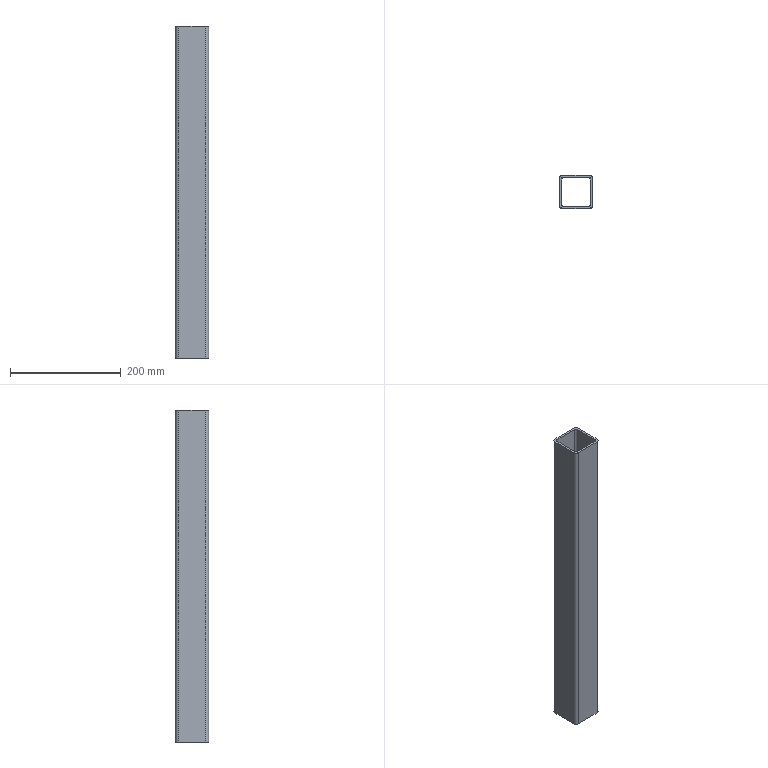Part | SolidWorks | features Fillet 2, Extrusion 1 | 1 solid | 18 faces | box 60 x 60 x 600 mm | volume 523694 mm3 | plane 10 | cylinder 8 | commonest cylinder face diameters 6 x4 12 x4
STEP:
#1=CARTESIAN_POINT('',(-24.,-30.,600.));
#2=VERTEX_POINT('',#1);
#3=CARTESIAN_POINT('',(24.,-30.,600.));
#4=VERTEX_POINT('',#3);
#5=CARTESIAN_POINT('',(-30.,-30.,600.));
#6=DIRECTION('',(1.,0.,0.));
#7=VECTOR('',#6,1000.);
#8=LINE('',#5,#7);
#9=EDGE_CURVE('',#2,#4,#8,.T.);
#10=ORIENTED_EDGE('',*,*,#9,.T.);
#11=CARTESIAN_POINT('',(30.,-24.,600.));
#12=VERTEX_POINT('',#11);
#13=CARTESIAN_POINT('',(24.,-24.,600.));
#14=DIRECTION('',(0.,0.,1.));
#15=DIRECTION('',(-1.,0.,0.));
#16=AXIS2_PLACEMENT_3D('',#13,#14,#15);
#17=CIRCLE('',#16,6.);
#18=EDGE_CURVE('',#4,#12,#17,.T.);
#19=ORIENTED_EDGE('',*,*,#18,.T.);
#20=CARTESIAN_POINT('',(30.,24.,600.));
#21=VERTEX_POINT('',#20);
#22=CARTESIAN_POINT('',(30.,-30.,600.));
#23=DIRECTION('',(0.,1.,0.));
#24=VECTOR('',#23,1000.);
#25=LINE('',#22,#24);
#26=EDGE_CURVE('',#12,#21,#25,.T.);
#27=ORIENTED_EDGE('',*,*,#26,.T.);
#28=CARTESIAN_POINT('',(24.,30.,600.));
#29=VERTEX_POINT('',#28);
#30=CARTESIAN_POINT('',(24.,24.,600.));
#31=DIRECTION('',(0.,0.,1.));
#32=DIRECTION('',(-1.,0.,0.));
#33=AXIS2_PLACEMENT_3D('',#30,#31,#32);
#34=CIRCLE('',#33,6.);
#35=EDGE_CURVE('',#21,#29,#34,.T.);
#36=ORIENTED_EDGE('',*,*,#35,.T.);
#37=CARTESIAN_POINT('',(-24.,30.,600.));
#38=VERTEX_POINT('',#37);
#39=CARTESIAN_POINT('',(-30.,30.,600.));
#40=DIRECTION('',(-1.,0.,0.));
#41=VECTOR('',#40,1000.);
#42=LINE('',#39,#41);
#43=EDGE_CURVE('',#29,#38,#42,.T.);
#44=ORIENTED_EDGE('',*,*,#43,.T.);
#45=CARTESIAN_POINT('',(-30.,24.,600.));
#46=VERTEX_POINT('',#45);
#47=CARTESIAN_POINT('',(-24.,24.,600.));
#48=DIRECTION('',(0.,0.,1.));
#49=DIRECTION('',(-1.,0.,0.));
#50=AXIS2_PLACEMENT_3D('',#47,#48,#49);
#51=CIRCLE('',#50,6.);
#52=EDGE_CURVE('',#38,#46,#51,.T.);
#53=ORIENTED_EDGE('',*,*,#52,.T.);
#54=CARTESIAN_POINT('',(-30.,-24.,600.));
#55=VERTEX_POINT('',#54);
#56=CARTESIAN_POINT('',(-30.,-30.,600.));
#57=DIRECTION('',(0.,-1.,0.));
#58=VECTOR('',#57,1000.);
#59=LINE('',#56,#58);
#60=EDGE_CURVE('',#46,#55,#59,.T.);
#61=ORIENTED_EDGE('',*,*,#60,.T.);
#62=CARTESIAN_POINT('',(-24.,-24.,600.));
#63=DIRECTION('',(0.,0.,1.));
#64=DIRECTION('',(-1.,0.,0.));
#65=AXIS2_PLACEMENT_3D('',#62,#63,#64);
#66=CIRCLE('',#65,6.);
#67=EDGE_CURVE('',#55,#2,#66,.T.);
#68=ORIENTED_EDGE('',*,*,#67,.T.);
#69=EDGE_LOOP('',(#10,#19,#27,#36,#44,#53,#61,#68));
#70=FACE_OUTER_BOUND('',#69,.T.);
#71=CARTESIAN_POINT('',(26.,-23.,600.));
#72=VERTEX_POINT('',#71);
#73=CARTESIAN_POINT('',(26.,23.,600.));
#74=VERTEX_POINT('',#73);
#75=CARTESIAN_POINT('',(26.,-26.,600.));
#76=DIRECTION('',(0.,1.,0.));
#77=VECTOR('',#76,1000.);
#78=LINE('',#75,#77);
#79=EDGE_CURVE('',#72,#74,#78,.T.);
#80=ORIENTED_EDGE('',*,*,#79,.F.);
#81=CARTESIAN_POINT('',(23.,-26.,600.));
#82=VERTEX_POINT('',#81);
#83=CARTESIAN_POINT('',(23.,-23.,600.));
#84=DIRECTION('',(0.,0.,-1.));
#85=DIRECTION('',(-1.,0.,0.));
#86=AXIS2_PLACEMENT_3D('',#83,#84,#85);
#87=CIRCLE('',#86,3.);
#88=EDGE_CURVE('',#72,#82,#87,.T.);
#89=ORIENTED_EDGE('',*,*,#88,.T.);
#90=CARTESIAN_POINT('',(-23.,-26.,600.));
#91=VERTEX_POINT('',#90);
#92=CARTESIAN_POINT('',(-26.,-26.,600.));
#93=DIRECTION('',(1.,0.,0.));
#94=VECTOR('',#93,1000.);
#95=LINE('',#92,#94);
#96=EDGE_CURVE('',#91,#82,#95,.T.);
#97=ORIENTED_EDGE('',*,*,#96,.F.);
#98=CARTESIAN_POINT('',(-26.,-23.,600.));
#99=VERTEX_POINT('',#98);
#100=CARTESIAN_POINT('',(-23.,-23.,600.));
#101=DIRECTION('',(0.,0.,-1.));
#102=DIRECTION('',(-1.,0.,0.));
#103=AXIS2_PLACEMENT_3D('',#100,#101,#102);
#104=CIRCLE('',#103,3.);
#105=EDGE_CURVE('',#91,#99,#104,.T.);
#106=ORIENTED_EDGE('',*,*,#105,.T.);
#107=CARTESIAN_POINT('',(-26.,23.,600.));
#108=VERTEX_POINT('',#107);
#109=CARTESIAN_POINT('',(-26.,-26.,600.));
#110=DIRECTION('',(0.,-1.,0.));
#111=VECTOR('',#110,1000.);
#112=LINE('',#109,#111);
#113=EDGE_CURVE('',#108,#99,#112,.T.);
#114=ORIENTED_EDGE('',*,*,#113,.F.);
#115=CARTESIAN_POINT('',(-23.,26.,600.));
#116=VERTEX_POINT('',#115);
#117=CARTESIAN_POINT('',(-23.,23.,600.));
#118=DIRECTION('',(0.,0.,-1.));
#119=DIRECTION('',(-1.,0.,0.));
#120=AXIS2_PLACEMENT_3D('',#117,#118,#119);
#121=CIRCLE('',#120,3.);
#122=EDGE_CURVE('',#108,#116,#121,.T.);
#123=ORIENTED_EDGE('',*,*,#122,.T.);
#124=CARTESIAN_POINT('',(23.,26.,600.));
#125=VERTEX_POINT('',#124);
#126=CARTESIAN_POINT('',(-26.,26.,600.));
#127=DIRECTION('',(-1.,0.,0.));
#128=VECTOR('',#127,1000.);
#129=LINE('',#126,#128);
#130=EDGE_CURVE('',#125,#116,#129,.T.);
#131=ORIENTED_EDGE('',*,*,#130,.F.);
#132=CARTESIAN_POINT('',(23.,23.,600.));
#133=DIRECTION('',(0.,0.,-1.));
#134=DIRECTION('',(-1.,0.,0.));
#135=AXIS2_PLACEMENT_3D('',#132,#133,#134);
#136=CIRCLE('',#135,3.);
#137=EDGE_CURVE('',#125,#74,#136,.T.);
#138=ORIENTED_EDGE('',*,*,#137,.T.);
#139=EDGE_LOOP('',(#80,#89,#97,#106,#114,#123,#131,#138));
#140=FACE_BOUND('',#139,.T.);
#141=CARTESIAN_POINT('',(0.,0.,600.));
#142=DIRECTION('',(0.,0.,-1.));
#143=DIRECTION('',(-1.,0.,0.));
#144=AXIS2_PLACEMENT_3D('',#141,#142,#143);
#145=PLANE('',#144);
#146=ADVANCED_FACE('',(#70,#140),#145,.F.);
#147=CARTESIAN_POINT('',(30.,-24.,0.));
#148=VERTEX_POINT('',#147);
#149=CARTESIAN_POINT('',(30.,24.,0.));
#150=VERTEX_POINT('',#149);
#151=CARTESIAN_POINT('',(30.,-30.,0.));
#152=DIRECTION('',(0.,1.,0.));
#153=VECTOR('',#152,1000.);
#154=LINE('',#151,#153);
#155=EDGE_CURVE('',#148,#150,#154,.T.);
#156=ORIENTED_EDGE('',*,*,#155,.F.);
#157=CARTESIAN_POINT('',(24.,-30.,0.));
#158=VERTEX_POINT('',#157);
#159=CARTESIAN_POINT('',(24.,-24.,0.));
#160=DIRECTION('',(0.,0.,-1.));
#161=DIRECTION('',(-1.,0.,0.));
#162=AXIS2_PLACEMENT_3D('',#159,#160,#161);
#163=CIRCLE('',#162,6.);
#164=EDGE_CURVE('',#148,#158,#163,.T.);
#165=ORIENTED_EDGE('',*,*,#164,.T.);
#166=CARTESIAN_POINT('',(-24.,-30.,0.));
#167=VERTEX_POINT('',#166);
#168=CARTESIAN_POINT('',(-30.,-30.,0.));
#169=DIRECTION('',(1.,0.,0.));
#170=VECTOR('',#169,1000.);
#171=LINE('',#168,#170);
#172=EDGE_CURVE('',#167,#158,#171,.T.);
#173=ORIENTED_EDGE('',*,*,#172,.F.);
#174=CARTESIAN_POINT('',(-30.,-24.,0.));
#175=VERTEX_POINT('',#174);
#176=CARTESIAN_POINT('',(-24.,-24.,0.));
#177=DIRECTION('',(0.,0.,-1.));
#178=DIRECTION('',(-1.,0.,0.));
#179=AXIS2_PLACEMENT_3D('',#176,#177,#178);
#180=CIRCLE('',#179,6.);
#181=EDGE_CURVE('',#167,#175,#180,.T.);
#182=ORIENTED_EDGE('',*,*,#181,.T.);
#183=CARTESIAN_POINT('',(-30.,24.,0.));
#184=VERTEX_POINT('',#183);
#185=CARTESIAN_POINT('',(-30.,-30.,0.));
#186=DIRECTION('',(0.,-1.,0.));
#187=VECTOR('',#186,1000.);
#188=LINE('',#185,#187);
#189=EDGE_CURVE('',#184,#175,#188,.T.);
#190=ORIENTED_EDGE('',*,*,#189,.F.);
#191=CARTESIAN_POINT('',(-24.,30.,0.));
#192=VERTEX_POINT('',#191);
#193=CARTESIAN_POINT('',(-24.,24.,0.));
#194=DIRECTION('',(0.,0.,-1.));
#195=DIRECTION('',(-1.,0.,0.));
#196=AXIS2_PLACEMENT_3D('',#193,#194,#195);
#197=CIRCLE('',#196,6.);
#198=EDGE_CURVE('',#184,#192,#197,.T.);
#199=ORIENTED_EDGE('',*,*,#198,.T.);
#200=CARTESIAN_POINT('',(24.,30.,0.));
#201=VERTEX_POINT('',#200);
#202=CARTESIAN_POINT('',(-30.,30.,0.));
#203=DIRECTION('',(-1.,0.,0.));
#204=VECTOR('',#203,1000.);
#205=LINE('',#202,#204);
#206=EDGE_CURVE('',#201,#192,#205,.T.);
#207=ORIENTED_EDGE('',*,*,#206,.F.);
#208=CARTESIAN_POINT('',(24.,24.,0.));
#209=DIRECTION('',(0.,0.,-1.));
#210=DIRECTION('',(-1.,0.,0.));
#211=AXIS2_PLACEMENT_3D('',#208,#209,#210);
#212=CIRCLE('',#211,6.);
#213=EDGE_CURVE('',#201,#150,#212,.T.);
#214=ORIENTED_EDGE('',*,*,#213,.T.);
#215=EDGE_LOOP('',(#156,#165,#173,#182,#190,#199,#207,#214));
#216=FACE_OUTER_BOUND('',#215,.T.);
#217=CARTESIAN_POINT('',(-26.,23.,0.));
#218=VERTEX_POINT('',#217);
#219=CARTESIAN_POINT('',(-26.,-23.,0.));
#220=VERTEX_POINT('',#219);
#221=CARTESIAN_POINT('',(-26.,-26.,0.));
#222=DIRECTION('',(0.,-1.,0.));
#223=VECTOR('',#222,1000.);
#224=LINE('',#221,#223);
#225=EDGE_CURVE('',#218,#220,#224,.T.);
#226=ORIENTED_EDGE('',*,*,#225,.T.);
#227=CARTESIAN_POINT('',(-23.,-26.,0.));
#228=VERTEX_POINT('',#227);
#229=CARTESIAN_POINT('',(-23.,-23.,0.));
#230=DIRECTION('',(0.,0.,1.));
#231=DIRECTION('',(-1.,0.,0.));
#232=AXIS2_PLACEMENT_3D('',#229,#230,#231);
#233=CIRCLE('',#232,3.);
#234=EDGE_CURVE('',#220,#228,#233,.T.);
#235=ORIENTED_EDGE('',*,*,#234,.T.);
#236=CARTESIAN_POINT('',(23.,-26.,0.));
#237=VERTEX_POINT('',#236);
#238=CARTESIAN_POINT('',(-26.,-26.,0.));
#239=DIRECTION('',(1.,0.,0.));
#240=VECTOR('',#239,1000.);
#241=LINE('',#238,#240);
#242=EDGE_CURVE('',#228,#237,#241,.T.);
#243=ORIENTED_EDGE('',*,*,#242,.T.);
#244=CARTESIAN_POINT('',(26.,-23.,0.));
#245=VERTEX_POINT('',#244);
#246=CARTESIAN_POINT('',(23.,-23.,0.));
#247=DIRECTION('',(0.,0.,1.));
#248=DIRECTION('',(-1.,0.,0.));
#249=AXIS2_PLACEMENT_3D('',#246,#247,#248);
#250=CIRCLE('',#249,3.);
#251=EDGE_CURVE('',#237,#245,#250,.T.);
#252=ORIENTED_EDGE('',*,*,#251,.T.);
#253=CARTESIAN_POINT('',(26.,23.,0.));
#254=VERTEX_POINT('',#253);
#255=CARTESIAN_POINT('',(26.,-26.,0.));
#256=DIRECTION('',(0.,1.,0.));
#257=VECTOR('',#256,1000.);
#258=LINE('',#255,#257);
#259=EDGE_CURVE('',#245,#254,#258,.T.);
#260=ORIENTED_EDGE('',*,*,#259,.T.);
#261=CARTESIAN_POINT('',(23.,26.,0.));
#262=VERTEX_POINT('',#261);
#263=CARTESIAN_POINT('',(23.,23.,0.));
#264=DIRECTION('',(0.,0.,1.));
#265=DIRECTION('',(-1.,0.,0.));
#266=AXIS2_PLACEMENT_3D('',#263,#264,#265);
#267=CIRCLE('',#266,3.);
#268=EDGE_CURVE('',#254,#262,#267,.T.);
#269=ORIENTED_EDGE('',*,*,#268,.T.);
#270=CARTESIAN_POINT('',(-23.,26.,0.));
#271=VERTEX_POINT('',#270);
#272=CARTESIAN_POINT('',(-26.,26.,0.));
#273=DIRECTION('',(-1.,0.,0.));
#274=VECTOR('',#273,1000.);
#275=LINE('',#272,#274);
#276=EDGE_CURVE('',#262,#271,#275,.T.);
#277=ORIENTED_EDGE('',*,*,#276,.T.);
#278=CARTESIAN_POINT('',(-23.,23.,0.));
#279=DIRECTION('',(0.,0.,1.));
#280=DIRECTION('',(-1.,0.,0.));
#281=AXIS2_PLACEMENT_3D('',#278,#279,#280);
#282=CIRCLE('',#281,3.);
#283=EDGE_CURVE('',#271,#218,#282,.T.);
#284=ORIENTED_EDGE('',*,*,#283,.T.);
#285=EDGE_LOOP('',(#226,#235,#243,#252,#260,#269,#277,#284));
#286=FACE_BOUND('',#285,.T.);
#287=CARTESIAN_POINT('',(0.,0.,0.));
#288=DIRECTION('',(0.,0.,-1.));
#289=DIRECTION('',(-1.,0.,0.));
#290=AXIS2_PLACEMENT_3D('',#287,#288,#289);
#291=PLANE('',#290);
#292=ADVANCED_FACE('',(#216,#286),#291,.T.);
#293=ORIENTED_EDGE('',*,*,#26,.F.);
#294=CARTESIAN_POINT('',(30.,-24.,600.));
#295=DIRECTION('',(0.,0.,-1.));
#296=VECTOR('',#295,1000.);
#297=LINE('',#294,#296);
#298=EDGE_CURVE('',#12,#148,#297,.T.);
#299=ORIENTED_EDGE('',*,*,#298,.T.);
#300=ORIENTED_EDGE('',*,*,#155,.T.);
#301=CARTESIAN_POINT('',(30.,24.,600.));
#302=DIRECTION('',(0.,0.,1.));
#303=VECTOR('',#302,1000.);
#304=LINE('',#301,#303);
#305=EDGE_CURVE('',#150,#21,#304,.T.);
#306=ORIENTED_EDGE('',*,*,#305,.T.);
#307=EDGE_LOOP('',(#293,#299,#300,#306));
#308=FACE_OUTER_BOUND('',#307,.T.);
#309=CARTESIAN_POINT('',(30.,-30.,600.));
#310=DIRECTION('',(-1.,0.,0.));
#311=DIRECTION('',(0.,0.,1.));
#312=AXIS2_PLACEMENT_3D('',#309,#310,#311);
#313=PLANE('',#312);
#314=ADVANCED_FACE('',(#308),#313,.F.);
#315=ORIENTED_EDGE('',*,*,#43,.F.);
#316=CARTESIAN_POINT('',(24.,30.,600.));
#317=DIRECTION('',(0.,0.,-1.));
#318=VECTOR('',#317,1000.);
#319=LINE('',#316,#318);
#320=EDGE_CURVE('',#29,#201,#319,.T.);
#321=ORIENTED_EDGE('',*,*,#320,.T.);
#322=ORIENTED_EDGE('',*,*,#206,.T.);
#323=CARTESIAN_POINT('',(-24.,30.,600.));
#324=DIRECTION('',(0.,0.,1.));
#325=VECTOR('',#324,1000.);
#326=LINE('',#323,#325);
#327=EDGE_CURVE('',#192,#38,#326,.T.);
#328=ORIENTED_EDGE('',*,*,#327,.T.);
#329=EDGE_LOOP('',(#315,#321,#322,#328));
#330=FACE_OUTER_BOUND('',#329,.T.);
#331=CARTESIAN_POINT('',(-30.,30.,600.));
#332=DIRECTION('',(0.,-1.,0.));
#333=DIRECTION('',(0.,0.,-1.));
#334=AXIS2_PLACEMENT_3D('',#331,#332,#333);
#335=PLANE('',#334);
#336=ADVANCED_FACE('',(#330),#335,.F.);
#337=ORIENTED_EDGE('',*,*,#189,.T.);
#338=CARTESIAN_POINT('',(-30.,-24.,600.));
#339=DIRECTION('',(0.,0.,1.));
#340=VECTOR('',#339,1000.);
#341=LINE('',#338,#340);
#342=EDGE_CURVE('',#175,#55,#341,.T.);
#343=ORIENTED_EDGE('',*,*,#342,.T.);
#344=ORIENTED_EDGE('',*,*,#60,.F.);
#345=CARTESIAN_POINT('',(-30.,24.,600.));
#346=DIRECTION('',(0.,0.,-1.));
#347=VECTOR('',#346,1000.);
#348=LINE('',#345,#347);
#349=EDGE_CURVE('',#46,#184,#348,.T.);
#350=ORIENTED_EDGE('',*,*,#349,.T.);
#351=EDGE_LOOP('',(#337,#343,#344,#350));
#352=FACE_OUTER_BOUND('',#351,.T.);
#353=CARTESIAN_POINT('',(-30.,-30.,600.));
#354=DIRECTION('',(1.,0.,0.));
#355=DIRECTION('',(0.,0.,-1.));
#356=AXIS2_PLACEMENT_3D('',#353,#354,#355);
#357=PLANE('',#356);
#358=ADVANCED_FACE('',(#352),#357,.F.);
#359=ORIENTED_EDGE('',*,*,#172,.T.);
#360=CARTESIAN_POINT('',(24.,-30.,600.));
#361=DIRECTION('',(0.,0.,1.));
#362=VECTOR('',#361,1000.);
#363=LINE('',#360,#362);
#364=EDGE_CURVE('',#158,#4,#363,.T.);
#365=ORIENTED_EDGE('',*,*,#364,.T.);
#366=ORIENTED_EDGE('',*,*,#9,.F.);
#367=CARTESIAN_POINT('',(-24.,-30.,600.));
#368=DIRECTION('',(0.,0.,-1.));
#369=VECTOR('',#368,1000.);
#370=LINE('',#367,#369);
#371=EDGE_CURVE('',#2,#167,#370,.T.);
#372=ORIENTED_EDGE('',*,*,#371,.T.);
#373=EDGE_LOOP('',(#359,#365,#366,#372));
#374=FACE_OUTER_BOUND('',#373,.T.);
#375=CARTESIAN_POINT('',(-30.,-30.,600.));
#376=DIRECTION('',(0.,1.,0.));
#377=DIRECTION('',(0.,0.,1.));
#378=AXIS2_PLACEMENT_3D('',#375,#376,#377);
#379=PLANE('',#378);
#380=ADVANCED_FACE('',(#374),#379,.F.);
#381=ORIENTED_EDGE('',*,*,#259,.F.);
#382=CARTESIAN_POINT('',(26.,-23.,600.));
#383=DIRECTION('',(0.,0.,1.));
#384=VECTOR('',#383,1000.);
#385=LINE('',#382,#384);
#386=EDGE_CURVE('',#245,#72,#385,.T.);
#387=ORIENTED_EDGE('',*,*,#386,.T.);
#388=ORIENTED_EDGE('',*,*,#79,.T.);
#389=CARTESIAN_POINT('',(26.,23.,0.));
#390=DIRECTION('',(0.,0.,-1.));
#391=VECTOR('',#390,1000.);
#392=LINE('',#389,#391);
#393=EDGE_CURVE('',#74,#254,#392,.T.);
#394=ORIENTED_EDGE('',*,*,#393,.T.);
#395=EDGE_LOOP('',(#381,#387,#388,#394));
#396=FACE_OUTER_BOUND('',#395,.T.);
#397=CARTESIAN_POINT('',(26.,-26.,600.));
#398=DIRECTION('',(-1.,0.,0.));
#399=DIRECTION('',(0.,0.,1.));
#400=AXIS2_PLACEMENT_3D('',#397,#398,#399);
#401=PLANE('',#400);
#402=ADVANCED_FACE('',(#396),#401,.T.);
#403=ORIENTED_EDGE('',*,*,#276,.F.);
#404=CARTESIAN_POINT('',(23.,26.,600.));
#405=DIRECTION('',(0.,0.,1.));
#406=VECTOR('',#405,1000.);
#407=LINE('',#404,#406);
#408=EDGE_CURVE('',#262,#125,#407,.T.);
#409=ORIENTED_EDGE('',*,*,#408,.T.);
#410=ORIENTED_EDGE('',*,*,#130,.T.);
#411=CARTESIAN_POINT('',(-23.,26.,0.));
#412=DIRECTION('',(0.,0.,-1.));
#413=VECTOR('',#412,1000.);
#414=LINE('',#411,#413);
#415=EDGE_CURVE('',#116,#271,#414,.T.);
#416=ORIENTED_EDGE('',*,*,#415,.T.);
#417=EDGE_LOOP('',(#403,#409,#410,#416));
#418=FACE_OUTER_BOUND('',#417,.T.);
#419=CARTESIAN_POINT('',(-26.,26.,600.));
#420=DIRECTION('',(0.,-1.,0.));
#421=DIRECTION('',(0.,0.,-1.));
#422=AXIS2_PLACEMENT_3D('',#419,#420,#421);
#423=PLANE('',#422);
#424=ADVANCED_FACE('',(#418),#423,.T.);
#425=ORIENTED_EDGE('',*,*,#113,.T.);
#426=CARTESIAN_POINT('',(-26.,-23.,0.));
#427=DIRECTION('',(0.,0.,-1.));
#428=VECTOR('',#427,1000.);
#429=LINE('',#426,#428);
#430=EDGE_CURVE('',#99,#220,#429,.T.);
#431=ORIENTED_EDGE('',*,*,#430,.T.);
#432=ORIENTED_EDGE('',*,*,#225,.F.);
#433=CARTESIAN_POINT('',(-26.,23.,600.));
#434=DIRECTION('',(0.,0.,1.));
#435=VECTOR('',#434,1000.);
#436=LINE('',#433,#435);
#437=EDGE_CURVE('',#218,#108,#436,.T.);
#438=ORIENTED_EDGE('',*,*,#437,.T.);
#439=EDGE_LOOP('',(#425,#431,#432,#438));
#440=FACE_OUTER_BOUND('',#439,.T.);
#441=CARTESIAN_POINT('',(-26.,-26.,600.));
#442=DIRECTION('',(1.,0.,0.));
#443=DIRECTION('',(0.,0.,-1.));
#444=AXIS2_PLACEMENT_3D('',#441,#442,#443);
#445=PLANE('',#444);
#446=ADVANCED_FACE('',(#440),#445,.T.);
#447=ORIENTED_EDGE('',*,*,#96,.T.);
#448=CARTESIAN_POINT('',(23.,-26.,0.));
#449=DIRECTION('',(0.,0.,-1.));
#450=VECTOR('',#449,1000.);
#451=LINE('',#448,#450);
#452=EDGE_CURVE('',#82,#237,#451,.T.);
#453=ORIENTED_EDGE('',*,*,#452,.T.);
#454=ORIENTED_EDGE('',*,*,#242,.F.);
#455=CARTESIAN_POINT('',(-23.,-26.,600.));
#456=DIRECTION('',(0.,0.,1.));
#457=VECTOR('',#456,1000.);
#458=LINE('',#455,#457);
#459=EDGE_CURVE('',#228,#91,#458,.T.);
#460=ORIENTED_EDGE('',*,*,#459,.T.);
#461=EDGE_LOOP('',(#447,#453,#454,#460));
#462=FACE_OUTER_BOUND('',#461,.T.);
#463=CARTESIAN_POINT('',(-26.,-26.,600.));
#464=DIRECTION('',(0.,1.,0.));
#465=DIRECTION('',(0.,0.,1.));
#466=AXIS2_PLACEMENT_3D('',#463,#464,#465);
#467=PLANE('',#466);
#468=ADVANCED_FACE('',(#462),#467,.T.);
#469=ORIENTED_EDGE('',*,*,#18,.F.);
#470=ORIENTED_EDGE('',*,*,#364,.F.);
#471=ORIENTED_EDGE('',*,*,#164,.F.);
#472=ORIENTED_EDGE('',*,*,#298,.F.);
#473=EDGE_LOOP('',(#469,#470,#471,#472));
#474=FACE_OUTER_BOUND('',#473,.T.);
#475=CARTESIAN_POINT('',(24.,-24.,600.));
#476=DIRECTION('',(0.,0.,-1.));
#477=DIRECTION('',(-1.,0.,0.));
#478=AXIS2_PLACEMENT_3D('',#475,#476,#477);
#479=CYLINDRICAL_SURFACE('',#478,6.);
#480=ADVANCED_FACE('',(#474),#479,.T.);
#481=ORIENTED_EDGE('',*,*,#67,.F.);
#482=ORIENTED_EDGE('',*,*,#342,.F.);
#483=ORIENTED_EDGE('',*,*,#181,.F.);
#484=ORIENTED_EDGE('',*,*,#371,.F.);
#485=EDGE_LOOP('',(#481,#482,#483,#484));
#486=FACE_OUTER_BOUND('',#485,.T.);
#487=CARTESIAN_POINT('',(-24.,-24.,600.));
#488=DIRECTION('',(0.,0.,-1.));
#489=DIRECTION('',(-1.,0.,0.));
#490=AXIS2_PLACEMENT_3D('',#487,#488,#489);
#491=CYLINDRICAL_SURFACE('',#490,6.);
#492=ADVANCED_FACE('',(#486),#491,.T.);
#493=ORIENTED_EDGE('',*,*,#35,.F.);
#494=ORIENTED_EDGE('',*,*,#305,.F.);
#495=ORIENTED_EDGE('',*,*,#213,.F.);
#496=ORIENTED_EDGE('',*,*,#320,.F.);
#497=EDGE_LOOP('',(#493,#494,#495,#496));
#498=FACE_OUTER_BOUND('',#497,.T.);
#499=CARTESIAN_POINT('',(24.,24.,600.));
#500=DIRECTION('',(0.,0.,-1.));
#501=DIRECTION('',(-1.,0.,0.));
#502=AXIS2_PLACEMENT_3D('',#499,#500,#501);
#503=CYLINDRICAL_SURFACE('',#502,6.);
#504=ADVANCED_FACE('',(#498),#503,.T.);
#505=ORIENTED_EDGE('',*,*,#52,.F.);
#506=ORIENTED_EDGE('',*,*,#327,.F.);
#507=ORIENTED_EDGE('',*,*,#198,.F.);
#508=ORIENTED_EDGE('',*,*,#349,.F.);
#509=EDGE_LOOP('',(#505,#506,#507,#508));
#510=FACE_OUTER_BOUND('',#509,.T.);
#511=CARTESIAN_POINT('',(-24.,24.,600.));
#512=DIRECTION('',(0.,0.,-1.));
#513=DIRECTION('',(-1.,0.,0.));
#514=AXIS2_PLACEMENT_3D('',#511,#512,#513);
#515=CYLINDRICAL_SURFACE('',#514,6.);
#516=ADVANCED_FACE('',(#510),#515,.T.);
#517=ORIENTED_EDGE('',*,*,#88,.F.);
#518=ORIENTED_EDGE('',*,*,#386,.F.);
#519=ORIENTED_EDGE('',*,*,#251,.F.);
#520=ORIENTED_EDGE('',*,*,#452,.F.);
#521=EDGE_LOOP('',(#517,#518,#519,#520));
#522=FACE_OUTER_BOUND('',#521,.T.);
#523=CARTESIAN_POINT('',(23.,-23.,600.));
#524=DIRECTION('',(0.,0.,1.));
#525=DIRECTION('',(1.,0.,0.));
#526=AXIS2_PLACEMENT_3D('',#523,#524,#525);
#527=CYLINDRICAL_SURFACE('',#526,3.);
#528=ADVANCED_FACE('',(#522),#527,.F.);
#529=ORIENTED_EDGE('',*,*,#105,.F.);
#530=ORIENTED_EDGE('',*,*,#459,.F.);
#531=ORIENTED_EDGE('',*,*,#234,.F.);
#532=ORIENTED_EDGE('',*,*,#430,.F.);
#533=EDGE_LOOP('',(#529,#530,#531,#532));
#534=FACE_OUTER_BOUND('',#533,.T.);
#535=CARTESIAN_POINT('',(-23.,-23.,600.));
#536=DIRECTION('',(0.,0.,1.));
#537=DIRECTION('',(1.,0.,0.));
#538=AXIS2_PLACEMENT_3D('',#535,#536,#537);
#539=CYLINDRICAL_SURFACE('',#538,3.);
#540=ADVANCED_FACE('',(#534),#539,.F.);
#541=ORIENTED_EDGE('',*,*,#137,.F.);
#542=ORIENTED_EDGE('',*,*,#408,.F.);
#543=ORIENTED_EDGE('',*,*,#268,.F.);
#544=ORIENTED_EDGE('',*,*,#393,.F.);
#545=EDGE_LOOP('',(#541,#542,#543,#544));
#546=FACE_OUTER_BOUND('',#545,.T.);
#547=CARTESIAN_POINT('',(23.,23.,600.));
#548=DIRECTION('',(0.,0.,1.));
#549=DIRECTION('',(1.,0.,0.));
#550=AXIS2_PLACEMENT_3D('',#547,#548,#549);
#551=CYLINDRICAL_SURFACE('',#550,3.);
#552=ADVANCED_FACE('',(#546),#551,.F.);
#553=ORIENTED_EDGE('',*,*,#122,.F.);
#554=ORIENTED_EDGE('',*,*,#437,.F.);
#555=ORIENTED_EDGE('',*,*,#283,.F.);
#556=ORIENTED_EDGE('',*,*,#415,.F.);
#557=EDGE_LOOP('',(#553,#554,#555,#556));
#558=FACE_OUTER_BOUND('',#557,.T.);
#559=CARTESIAN_POINT('',(-23.,23.,600.));
#560=DIRECTION('',(0.,0.,1.));
#561=DIRECTION('',(1.,0.,0.));
#562=AXIS2_PLACEMENT_3D('',#559,#560,#561);
#563=CYLINDRICAL_SURFACE('',#562,3.);
#564=ADVANCED_FACE('',(#558),#563,.F.);
#565=CLOSED_SHELL('',(#146,#292,#314,#336,#358,#380,#402,#424,#446,#468,#480,#492,#504,#516,#528,#540,#552,#564));
#566=MANIFOLD_SOLID_BREP('',#565);
#567=CARTESIAN_POINT('',(0.,0.,0.));
#568=DIRECTION('',(0.,0.,1.));
#569=DIRECTION('',(1.,0.,0.));
#570=AXIS2_PLACEMENT_3D('',#567,#568,#569);
#571=(LENGTH_UNIT()NAMED_UNIT(*)SI_UNIT(.MILLI.,.METRE.));
#572=UNCERTAINTY_MEASURE_WITH_UNIT(LENGTH_MEASURE(0.00001),#571,'','');
#573=(NAMED_UNIT(*)PLANE_ANGLE_UNIT()SI_UNIT($,.RADIAN.));
#574=(NAMED_UNIT(*)SI_UNIT($,.STERADIAN.)SOLID_ANGLE_UNIT());
#575=(GEOMETRIC_REPRESENTATION_CONTEXT(3)GLOBAL_UNCERTAINTY_ASSIGNED_CONTEXT((#572))GLOBAL_UNIT_ASSIGNED_CONTEXT((#571,#573,#574))REPRESENTATION_CONTEXT('',''));
#576=ADVANCED_BREP_SHAPE_REPRESENTATION('',(#566,#570),#575);